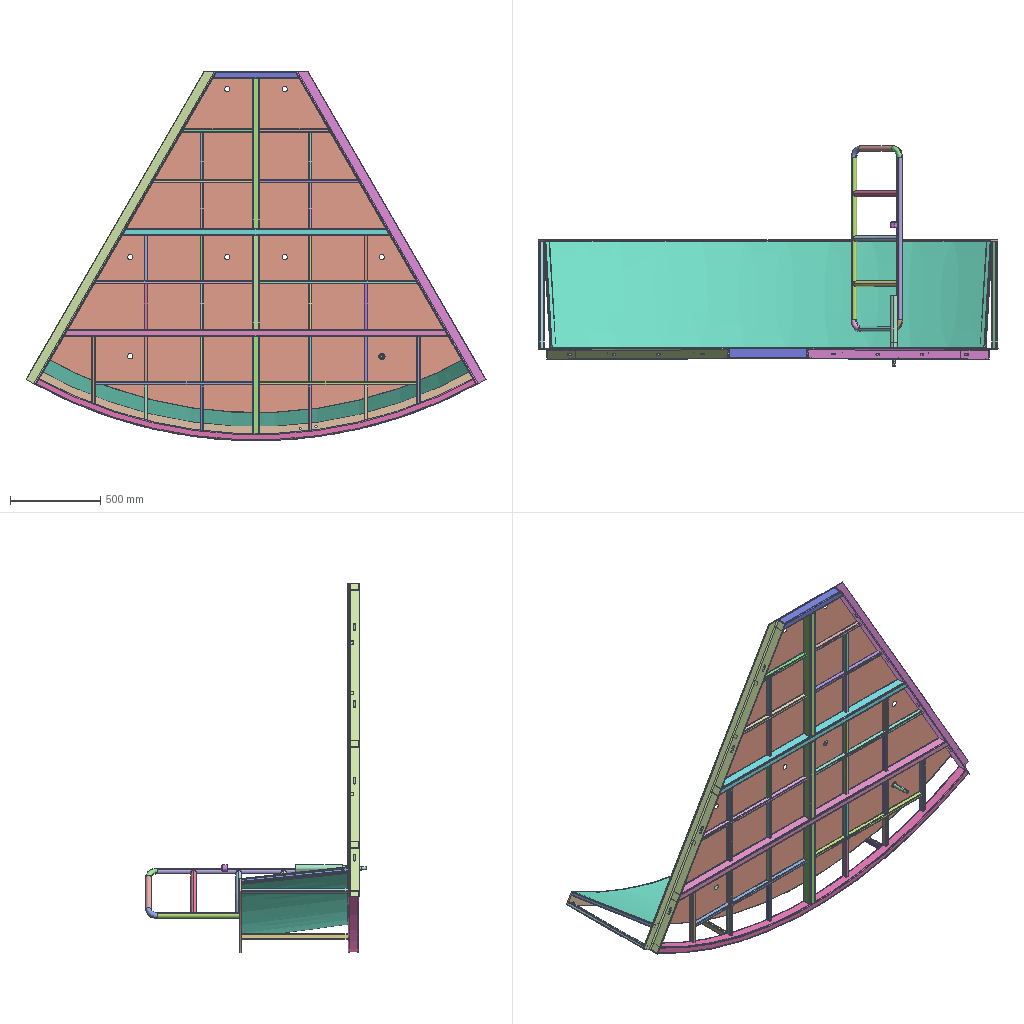Assembly | SolidWorks | 8 different items | 8 placed | box 2550 x 1224 x 2050 mm
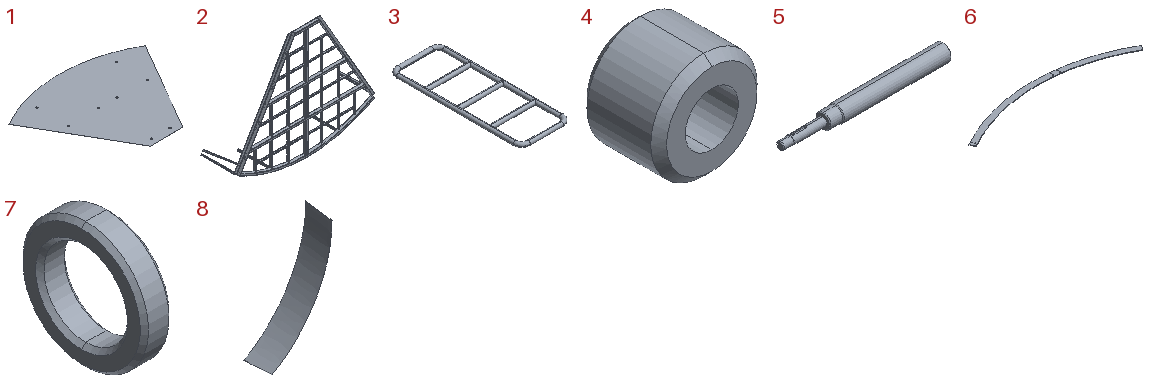Parts list (item | quantity | size | volume | features):
1 | x1 | 2393 x 1893 x 1 mm | 2848544 mm3 | features FlatPattern 1, HoleWzd 1, SMBaseFlange 1, SheetMetal 1
2 | x1 | 2550 x 655 x 2050 mm | 9987887 mm3 | features WeldCornerFeat 14, WeldMemberFeat 6, ICE 2, MirrorSolid 1, WeldmentFeature 1
3 | x1 | 387 x 1032 x 32 mm | 682567 mm3 | features WeldMemberFeat 1, WeldmentFeature 1
4 | x1 | 40 x 30 x 40 mm | 27200 mm3 | features Chamfer 1, Extrusion 1
5 | x1 | 393 x 40 x 40 mm | 386098 mm3 | features ICE 2, Chamfer 1, Revolution 1
6 | x1 | 2550 x 410.917 x 8 mm | 1676789 mm3 | features Extrusion 1, HoleWzd 1
7 | x1 | 6.9 x 30 x 30 mm | 2553 mm3 | features Chamfer 1, Extrusion 1
8 | x1 | 1273 x 598.126 x 2139 mm | 1534665 mm3 | features FlatPattern 1, ICE 1, LoftedBend 1, SheetMetal 1
Mates (type | each side: item.copy, entity, surface, feature):
Tangent | 3.1 face cylinder GB/T 6728-2002 round tube 32 × 2-example.com(1) | 5.1 face cylinder Revolve1
DistanceDim | 4.1 face plane Boss-Extrude1 | 5.1 face plane Revolve1
Concentric | 4.1 face cylinder Boss-Extrude1 | 5.1 face cylinder Revolve1
Coincident | 1.1 face plane Base-Flange1 | 2.1 face plane Cold-formed square hollow steel (GB/T 6728-2002) 60×40×3(1) | 2 times
Coincident | 2.1 face plane Hot-rolled equal-leg angle steel (GB/T 9787-1988) 63×6(1) | 8.1 plane
Coincident | 2.1 face plane Cold-formed square hollow steel (GB/T 6728-2002) 30×20×2(2) | 8.1 face plane Cut-Extrude2
Concentric | 5.1 face cylinder Revolve1 | 1.1 face cylinder Ø30 diameter hole1
Coincident | 5.1 face plane Revolve1 | 1.1 face plane Base-Flange1
Concentric | 2.1 face cylinder Cold-formed square hollow steel (GB/T 6728-2002) 60×40×3(1) | 6.1 face cylinder Boss-Extrude1
Coincident | 2.1 face plane Trim/extend18 | 6.1 face plane Boss-Extrude1
Parallel | 2.1 face plane Mirror1 | 6.1 face plane Boss-Extrude1
Concentric | 4.1 face cylinder Boss-Extrude1 | 7.1 face cylinder Boss-Extrude1
Coincident | 4.1 face plane Boss-Extrude1 | 7.1 face plane Boss-Extrude1
Coincident | 1.1 face plane Base-Flange1 | 2.1 face plane Hot-rolled equal-leg angle steel (GB/T 9787-1988) 63×6(1)
Coordinate | 2.1 select_type:25 | assembly select_type:11
Coincident | 2.1 face plane Mirror1 | 8.1 face plane Freeform bend1